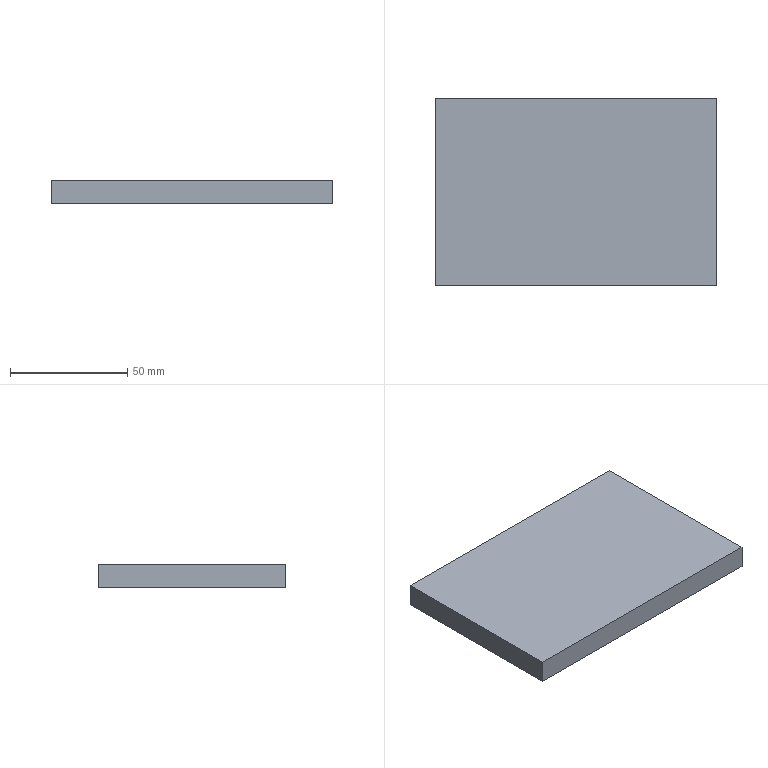Part | SolidWorks | features ICE 4, Extrusion 1 | 1 solid | 6 faces | box 120 x 80 x 10 mm | volume 96000 mm3 | plane 6
STEP:
#1=CARTESIAN_POINT('',(-60.,40.,0.));
#2=VERTEX_POINT('',#1);
#3=CARTESIAN_POINT('',(60.,40.,0.));
#4=VERTEX_POINT('',#3);
#5=CARTESIAN_POINT('',(-60.,40.,0.));
#6=DIRECTION('',(1.,0.,0.));
#7=VECTOR('',#6,1000.);
#8=LINE('',#5,#7);
#9=EDGE_CURVE('',#2,#4,#8,.T.);
#10=ORIENTED_EDGE('',*,*,#9,.T.);
#11=CARTESIAN_POINT('',(60.,40.,-10.));
#12=VERTEX_POINT('',#11);
#13=CARTESIAN_POINT('',(60.,40.,-10.));
#14=DIRECTION('',(0.,0.,1.));
#15=VECTOR('',#14,1000.);
#16=LINE('',#13,#15);
#17=EDGE_CURVE('',#12,#4,#16,.T.);
#18=ORIENTED_EDGE('',*,*,#17,.F.);
#19=CARTESIAN_POINT('',(-60.,40.,-10.));
#20=VERTEX_POINT('',#19);
#21=CARTESIAN_POINT('',(-60.,40.,-10.));
#22=DIRECTION('',(1.,0.,0.));
#23=VECTOR('',#22,1000.);
#24=LINE('',#21,#23);
#25=EDGE_CURVE('',#20,#12,#24,.T.);
#26=ORIENTED_EDGE('',*,*,#25,.F.);
#27=CARTESIAN_POINT('',(-60.,40.,-10.));
#28=DIRECTION('',(0.,0.,1.));
#29=VECTOR('',#28,1000.);
#30=LINE('',#27,#29);
#31=EDGE_CURVE('',#20,#2,#30,.T.);
#32=ORIENTED_EDGE('',*,*,#31,.T.);
#33=EDGE_LOOP('',(#10,#18,#26,#32));
#34=FACE_OUTER_BOUND('',#33,.T.);
#35=CARTESIAN_POINT('',(-60.,40.,-10.));
#36=DIRECTION('',(0.,-1.,0.));
#37=DIRECTION('',(1.,0.,0.));
#38=AXIS2_PLACEMENT_3D('',#35,#36,#37);
#39=PLANE('',#38);
#40=ADVANCED_FACE('',(#34),#39,.F.);
#41=CARTESIAN_POINT('',(60.,-40.,0.));
#42=VERTEX_POINT('',#41);
#43=CARTESIAN_POINT('',(60.,40.,0.));
#44=DIRECTION('',(0.,-1.,0.));
#45=VECTOR('',#44,1000.);
#46=LINE('',#43,#45);
#47=EDGE_CURVE('',#4,#42,#46,.T.);
#48=ORIENTED_EDGE('',*,*,#47,.T.);
#49=CARTESIAN_POINT('',(60.,-40.,-10.));
#50=VERTEX_POINT('',#49);
#51=CARTESIAN_POINT('',(60.,-40.,-10.));
#52=DIRECTION('',(0.,0.,1.));
#53=VECTOR('',#52,1000.);
#54=LINE('',#51,#53);
#55=EDGE_CURVE('',#50,#42,#54,.T.);
#56=ORIENTED_EDGE('',*,*,#55,.F.);
#57=CARTESIAN_POINT('',(60.,40.,-10.));
#58=DIRECTION('',(0.,-1.,0.));
#59=VECTOR('',#58,1000.);
#60=LINE('',#57,#59);
#61=EDGE_CURVE('',#12,#50,#60,.T.);
#62=ORIENTED_EDGE('',*,*,#61,.F.);
#63=ORIENTED_EDGE('',*,*,#17,.T.);
#64=EDGE_LOOP('',(#48,#56,#62,#63));
#65=FACE_OUTER_BOUND('',#64,.T.);
#66=CARTESIAN_POINT('',(60.,40.,-10.));
#67=DIRECTION('',(-1.,0.,0.));
#68=DIRECTION('',(0.,0.,1.));
#69=AXIS2_PLACEMENT_3D('',#66,#67,#68);
#70=PLANE('',#69);
#71=ADVANCED_FACE('',(#65),#70,.F.);
#72=CARTESIAN_POINT('',(-60.,-40.,0.));
#73=VERTEX_POINT('',#72);
#74=CARTESIAN_POINT('',(60.,-40.,0.));
#75=DIRECTION('',(-1.,0.,0.));
#76=VECTOR('',#75,1000.);
#77=LINE('',#74,#76);
#78=EDGE_CURVE('',#42,#73,#77,.T.);
#79=ORIENTED_EDGE('',*,*,#78,.T.);
#80=CARTESIAN_POINT('',(-60.,-40.,-10.));
#81=VERTEX_POINT('',#80);
#82=CARTESIAN_POINT('',(-60.,-40.,-10.));
#83=DIRECTION('',(0.,0.,1.));
#84=VECTOR('',#83,1000.);
#85=LINE('',#82,#84);
#86=EDGE_CURVE('',#81,#73,#85,.T.);
#87=ORIENTED_EDGE('',*,*,#86,.F.);
#88=CARTESIAN_POINT('',(60.,-40.,-10.));
#89=DIRECTION('',(-1.,0.,0.));
#90=VECTOR('',#89,1000.);
#91=LINE('',#88,#90);
#92=EDGE_CURVE('',#50,#81,#91,.T.);
#93=ORIENTED_EDGE('',*,*,#92,.F.);
#94=ORIENTED_EDGE('',*,*,#55,.T.);
#95=EDGE_LOOP('',(#79,#87,#93,#94));
#96=FACE_OUTER_BOUND('',#95,.T.);
#97=CARTESIAN_POINT('',(60.,-40.,-10.));
#98=DIRECTION('',(0.,1.,0.));
#99=DIRECTION('',(-1.,0.,0.));
#100=AXIS2_PLACEMENT_3D('',#97,#98,#99);
#101=PLANE('',#100);
#102=ADVANCED_FACE('',(#96),#101,.F.);
#103=CARTESIAN_POINT('',(-60.,-40.,0.));
#104=DIRECTION('',(0.,1.,0.));
#105=VECTOR('',#104,1000.);
#106=LINE('',#103,#105);
#107=EDGE_CURVE('',#73,#2,#106,.T.);
#108=ORIENTED_EDGE('',*,*,#107,.T.);
#109=ORIENTED_EDGE('',*,*,#31,.F.);
#110=CARTESIAN_POINT('',(-60.,-40.,-10.));
#111=DIRECTION('',(0.,1.,0.));
#112=VECTOR('',#111,1000.);
#113=LINE('',#110,#112);
#114=EDGE_CURVE('',#81,#20,#113,.T.);
#115=ORIENTED_EDGE('',*,*,#114,.F.);
#116=ORIENTED_EDGE('',*,*,#86,.T.);
#117=EDGE_LOOP('',(#108,#109,#115,#116));
#118=FACE_OUTER_BOUND('',#117,.T.);
#119=CARTESIAN_POINT('',(-60.,-40.,-10.));
#120=DIRECTION('',(1.,0.,0.));
#121=DIRECTION('',(0.,1.,0.));
#122=AXIS2_PLACEMENT_3D('',#119,#120,#121);
#123=PLANE('',#122);
#124=ADVANCED_FACE('',(#118),#123,.F.);
#125=ORIENTED_EDGE('',*,*,#25,.T.);
#126=ORIENTED_EDGE('',*,*,#61,.T.);
#127=ORIENTED_EDGE('',*,*,#92,.T.);
#128=ORIENTED_EDGE('',*,*,#114,.T.);
#129=EDGE_LOOP('',(#125,#126,#127,#128));
#130=FACE_OUTER_BOUND('',#129,.T.);
#131=CARTESIAN_POINT('',(0.,0.,-10.));
#132=DIRECTION('',(0.,0.,-1.));
#133=DIRECTION('',(-1.,0.,0.));
#134=AXIS2_PLACEMENT_3D('',#131,#132,#133);
#135=PLANE('',#134);
#136=ADVANCED_FACE('',(#130),#135,.T.);
#137=ORIENTED_EDGE('',*,*,#9,.F.);
#138=ORIENTED_EDGE('',*,*,#107,.F.);
#139=ORIENTED_EDGE('',*,*,#78,.F.);
#140=ORIENTED_EDGE('',*,*,#47,.F.);
#141=EDGE_LOOP('',(#137,#138,#139,#140));
#142=FACE_OUTER_BOUND('',#141,.T.);
#143=CARTESIAN_POINT('',(0.,0.,0.));
#144=DIRECTION('',(0.,0.,-1.));
#145=DIRECTION('',(-1.,0.,0.));
#146=AXIS2_PLACEMENT_3D('',#143,#144,#145);
#147=PLANE('',#146);
#148=ADVANCED_FACE('',(#142),#147,.F.);
#149=CLOSED_SHELL('',(#40,#71,#102,#124,#136,#148));
#150=MANIFOLD_SOLID_BREP('',#149);
#151=CARTESIAN_POINT('',(0.,0.,0.));
#152=DIRECTION('',(0.,0.,1.));
#153=DIRECTION('',(1.,0.,0.));
#154=AXIS2_PLACEMENT_3D('',#151,#152,#153);
#155=(LENGTH_UNIT()NAMED_UNIT(*)SI_UNIT(.MILLI.,.METRE.));
#156=UNCERTAINTY_MEASURE_WITH_UNIT(LENGTH_MEASURE(0.00001),#155,'','');
#157=(NAMED_UNIT(*)PLANE_ANGLE_UNIT()SI_UNIT($,.RADIAN.));
#158=(NAMED_UNIT(*)SI_UNIT($,.STERADIAN.)SOLID_ANGLE_UNIT());
#159=(GEOMETRIC_REPRESENTATION_CONTEXT(3)GLOBAL_UNCERTAINTY_ASSIGNED_CONTEXT((#156))GLOBAL_UNIT_ASSIGNED_CONTEXT((#155,#157,#158))REPRESENTATION_CONTEXT('',''));
#160=ADVANCED_BREP_SHAPE_REPRESENTATION('',(#150,#154),#159);